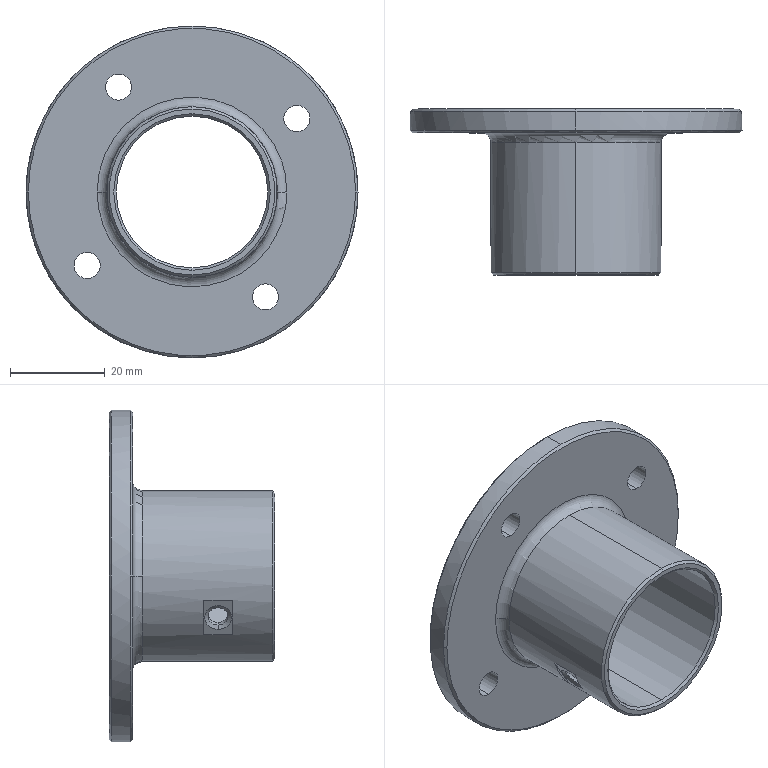Part | STEP file | Support base1 | 1 solid | 36 faces | box 70 x 35 x 70 mm | volume 21049 mm3 | cylinder 16 | cone 10 | plane 6 | torus 4 | commonest cylinder face diameters 5.5 x8 4.2 x2 32 x2 36 x2 70 x2